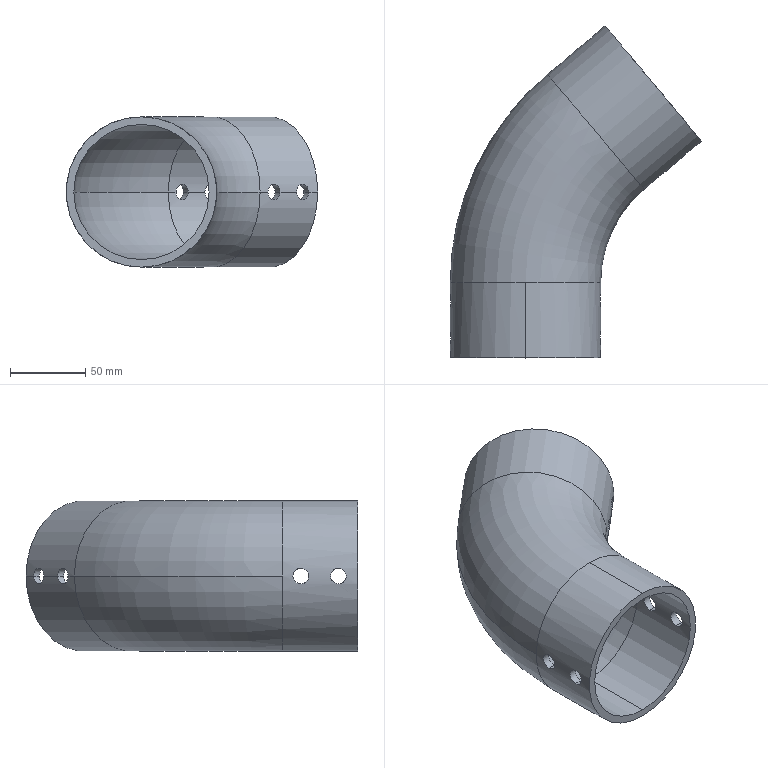Part | SolidWorks | features MirrorStock 1 | 1 solid | 30 faces | box 167.236 x 220.793 x 100 mm | volume 316350 mm3 | cylinder 24 | torus 4 | plane 2 | commonest cylinder face diameters 10.5 x16 90 x4 100 x4